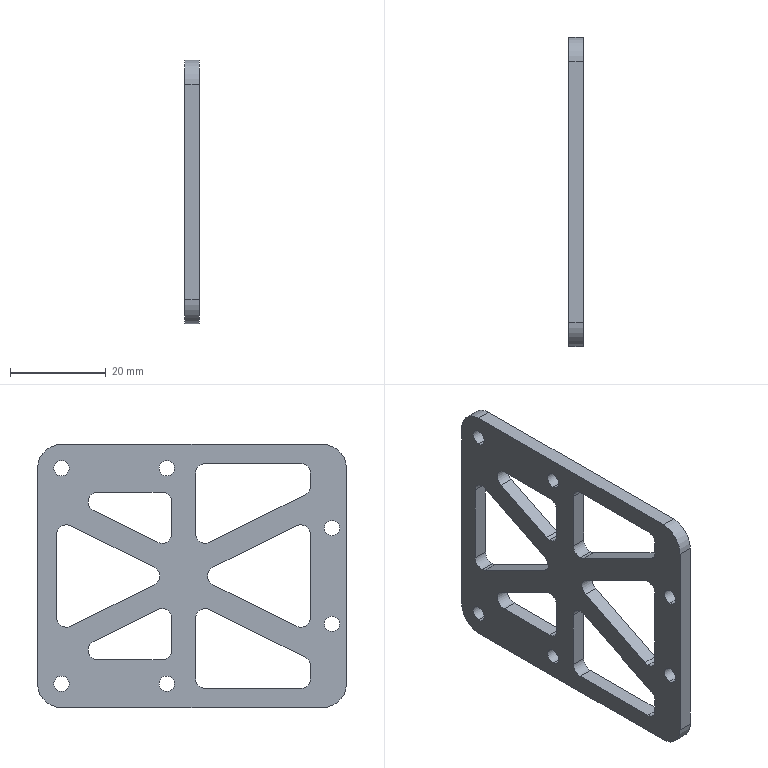Part | SolidWorks | features Fillet 2, ICE 2, Extrusion 1 | 1 solid | 66 faces | box 3 x 64.5 x 55 mm | volume 6303 mm3 | cylinder 40 | plane 26 | commonest cylinder face diameters 4 x24 3.2 x12 10 x4